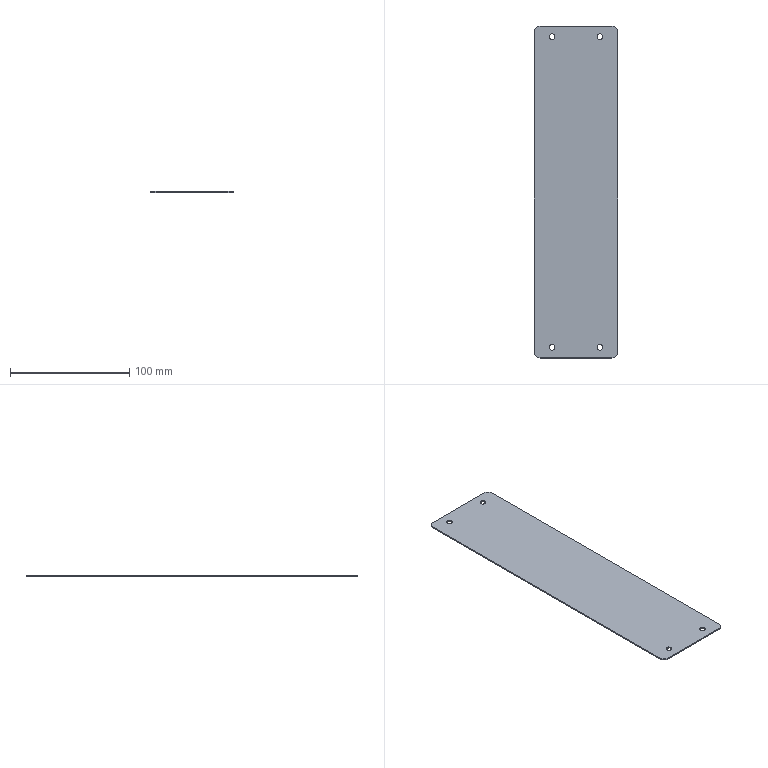Part | SolidWorks | features BreakCorner 1, FlatPattern 1, HoleWzd 1, SMBaseFlange 1, SheetMetal 1 | 1 solid | 18 faces | box 70 x 278 x 1 mm | volume 19366 mm3 | cylinder 12 | plane 6 | commonest cylinder face diameters 4.8 x8 10 x4
STEP:
#1=CARTESIAN_POINT('',(20.,127.6,0.));
#2=VERTEX_POINT('',#1);
#3=CARTESIAN_POINT('',(20.,132.4,0.));
#4=VERTEX_POINT('',#3);
#5=CARTESIAN_POINT('',(20.,130.,0.));
#6=DIRECTION('',(0.,0.,-1.));
#7=DIRECTION('',(0.,1.,0.));
#8=AXIS2_PLACEMENT_3D('',#5,#6,#7);
#9=CIRCLE('',#8,2.4);
#10=EDGE_CURVE('',#2,#4,#9,.T.);
#11=ORIENTED_EDGE('',*,*,#10,.F.);
#12=CARTESIAN_POINT('',(20.,127.6,-1.));
#13=VERTEX_POINT('',#12);
#14=CARTESIAN_POINT('',(20.,127.6,-1.));
#15=DIRECTION('',(0.,0.,-1.));
#16=VECTOR('',#15,1000.);
#17=LINE('',#14,#16);
#18=EDGE_CURVE('',#2,#13,#17,.T.);
#19=ORIENTED_EDGE('',*,*,#18,.T.);
#20=CARTESIAN_POINT('',(20.,132.4,-1.));
#21=VERTEX_POINT('',#20);
#22=CARTESIAN_POINT('',(20.,130.,-1.));
#23=DIRECTION('',(0.,0.,-1.));
#24=DIRECTION('',(0.,1.,0.));
#25=AXIS2_PLACEMENT_3D('',#22,#23,#24);
#26=CIRCLE('',#25,2.4);
#27=EDGE_CURVE('',#13,#21,#26,.T.);
#28=ORIENTED_EDGE('',*,*,#27,.T.);
#29=CARTESIAN_POINT('',(20.,132.4,-1.));
#30=DIRECTION('',(0.,0.,-1.));
#31=VECTOR('',#30,1000.);
#32=LINE('',#29,#31);
#33=EDGE_CURVE('',#4,#21,#32,.T.);
#34=ORIENTED_EDGE('',*,*,#33,.F.);
#35=EDGE_LOOP('',(#11,#19,#28,#34));
#36=FACE_OUTER_BOUND('',#35,.T.);
#37=CARTESIAN_POINT('',(20.,130.,-1.));
#38=DIRECTION('',(0.,0.,-1.));
#39=DIRECTION('',(0.,1.,0.));
#40=AXIS2_PLACEMENT_3D('',#37,#38,#39);
#41=CYLINDRICAL_SURFACE('',#40,2.4);
#42=ADVANCED_FACE('',(#36),#41,.F.);
#43=CARTESIAN_POINT('',(-20.,127.6,0.));
#44=VERTEX_POINT('',#43);
#45=CARTESIAN_POINT('',(-20.,132.4,0.));
#46=VERTEX_POINT('',#45);
#47=CARTESIAN_POINT('',(-20.,130.,0.));
#48=DIRECTION('',(0.,0.,-1.));
#49=DIRECTION('',(0.,1.,0.));
#50=AXIS2_PLACEMENT_3D('',#47,#48,#49);
#51=CIRCLE('',#50,2.4);
#52=EDGE_CURVE('',#44,#46,#51,.T.);
#53=ORIENTED_EDGE('',*,*,#52,.F.);
#54=CARTESIAN_POINT('',(-20.,127.6,-1.));
#55=VERTEX_POINT('',#54);
#56=CARTESIAN_POINT('',(-20.,127.6,-1.));
#57=DIRECTION('',(0.,0.,-1.));
#58=VECTOR('',#57,1000.);
#59=LINE('',#56,#58);
#60=EDGE_CURVE('',#44,#55,#59,.T.);
#61=ORIENTED_EDGE('',*,*,#60,.T.);
#62=CARTESIAN_POINT('',(-20.,132.4,-1.));
#63=VERTEX_POINT('',#62);
#64=CARTESIAN_POINT('',(-20.,130.,-1.));
#65=DIRECTION('',(0.,0.,-1.));
#66=DIRECTION('',(0.,1.,0.));
#67=AXIS2_PLACEMENT_3D('',#64,#65,#66);
#68=CIRCLE('',#67,2.4);
#69=EDGE_CURVE('',#55,#63,#68,.T.);
#70=ORIENTED_EDGE('',*,*,#69,.T.);
#71=CARTESIAN_POINT('',(-20.,132.4,-1.));
#72=DIRECTION('',(0.,0.,-1.));
#73=VECTOR('',#72,1000.);
#74=LINE('',#71,#73);
#75=EDGE_CURVE('',#46,#63,#74,.T.);
#76=ORIENTED_EDGE('',*,*,#75,.F.);
#77=EDGE_LOOP('',(#53,#61,#70,#76));
#78=FACE_OUTER_BOUND('',#77,.T.);
#79=CARTESIAN_POINT('',(-20.,130.,-1.));
#80=DIRECTION('',(0.,0.,-1.));
#81=DIRECTION('',(0.,1.,0.));
#82=AXIS2_PLACEMENT_3D('',#79,#80,#81);
#83=CYLINDRICAL_SURFACE('',#82,2.4);
#84=ADVANCED_FACE('',(#78),#83,.F.);
#85=CARTESIAN_POINT('',(20.,-132.4,0.));
#86=VERTEX_POINT('',#85);
#87=CARTESIAN_POINT('',(20.,-127.6,0.));
#88=VERTEX_POINT('',#87);
#89=CARTESIAN_POINT('',(20.,-130.,0.));
#90=DIRECTION('',(0.,0.,-1.));
#91=DIRECTION('',(0.,1.,0.));
#92=AXIS2_PLACEMENT_3D('',#89,#90,#91);
#93=CIRCLE('',#92,2.4);
#94=EDGE_CURVE('',#86,#88,#93,.T.);
#95=ORIENTED_EDGE('',*,*,#94,.F.);
#96=CARTESIAN_POINT('',(20.,-132.4,-1.));
#97=VERTEX_POINT('',#96);
#98=CARTESIAN_POINT('',(20.,-132.4,-1.));
#99=DIRECTION('',(0.,0.,-1.));
#100=VECTOR('',#99,1000.);
#101=LINE('',#98,#100);
#102=EDGE_CURVE('',#86,#97,#101,.T.);
#103=ORIENTED_EDGE('',*,*,#102,.T.);
#104=CARTESIAN_POINT('',(20.,-127.6,-1.));
#105=VERTEX_POINT('',#104);
#106=CARTESIAN_POINT('',(20.,-130.,-1.));
#107=DIRECTION('',(0.,0.,-1.));
#108=DIRECTION('',(0.,1.,0.));
#109=AXIS2_PLACEMENT_3D('',#106,#107,#108);
#110=CIRCLE('',#109,2.4);
#111=EDGE_CURVE('',#97,#105,#110,.T.);
#112=ORIENTED_EDGE('',*,*,#111,.T.);
#113=CARTESIAN_POINT('',(20.,-127.6,-1.));
#114=DIRECTION('',(0.,0.,-1.));
#115=VECTOR('',#114,1000.);
#116=LINE('',#113,#115);
#117=EDGE_CURVE('',#88,#105,#116,.T.);
#118=ORIENTED_EDGE('',*,*,#117,.F.);
#119=EDGE_LOOP('',(#95,#103,#112,#118));
#120=FACE_OUTER_BOUND('',#119,.T.);
#121=CARTESIAN_POINT('',(20.,-130.,-1.));
#122=DIRECTION('',(0.,0.,-1.));
#123=DIRECTION('',(0.,1.,0.));
#124=AXIS2_PLACEMENT_3D('',#121,#122,#123);
#125=CYLINDRICAL_SURFACE('',#124,2.4);
#126=ADVANCED_FACE('',(#120),#125,.F.);
#127=CARTESIAN_POINT('',(-20.,-132.4,0.));
#128=VERTEX_POINT('',#127);
#129=CARTESIAN_POINT('',(-20.,-127.6,0.));
#130=VERTEX_POINT('',#129);
#131=CARTESIAN_POINT('',(-20.,-130.,0.));
#132=DIRECTION('',(0.,0.,-1.));
#133=DIRECTION('',(0.,1.,0.));
#134=AXIS2_PLACEMENT_3D('',#131,#132,#133);
#135=CIRCLE('',#134,2.4);
#136=EDGE_CURVE('',#128,#130,#135,.T.);
#137=ORIENTED_EDGE('',*,*,#136,.F.);
#138=CARTESIAN_POINT('',(-20.,-132.4,-1.));
#139=VERTEX_POINT('',#138);
#140=CARTESIAN_POINT('',(-20.,-132.4,-1.));
#141=DIRECTION('',(0.,0.,-1.));
#142=VECTOR('',#141,1000.);
#143=LINE('',#140,#142);
#144=EDGE_CURVE('',#128,#139,#143,.T.);
#145=ORIENTED_EDGE('',*,*,#144,.T.);
#146=CARTESIAN_POINT('',(-20.,-127.6,-1.));
#147=VERTEX_POINT('',#146);
#148=CARTESIAN_POINT('',(-20.,-130.,-1.));
#149=DIRECTION('',(0.,0.,-1.));
#150=DIRECTION('',(0.,1.,0.));
#151=AXIS2_PLACEMENT_3D('',#148,#149,#150);
#152=CIRCLE('',#151,2.4);
#153=EDGE_CURVE('',#139,#147,#152,.T.);
#154=ORIENTED_EDGE('',*,*,#153,.T.);
#155=CARTESIAN_POINT('',(-20.,-127.6,-1.));
#156=DIRECTION('',(0.,0.,-1.));
#157=VECTOR('',#156,1000.);
#158=LINE('',#155,#157);
#159=EDGE_CURVE('',#130,#147,#158,.T.);
#160=ORIENTED_EDGE('',*,*,#159,.F.);
#161=EDGE_LOOP('',(#137,#145,#154,#160));
#162=FACE_OUTER_BOUND('',#161,.T.);
#163=CARTESIAN_POINT('',(-20.,-130.,-1.));
#164=DIRECTION('',(0.,0.,-1.));
#165=DIRECTION('',(0.,1.,0.));
#166=AXIS2_PLACEMENT_3D('',#163,#164,#165);
#167=CYLINDRICAL_SURFACE('',#166,2.4);
#168=ADVANCED_FACE('',(#162),#167,.F.);
#169=CARTESIAN_POINT('',(35.,-134.,-1.));
#170=VERTEX_POINT('',#169);
#171=CARTESIAN_POINT('',(35.,134.,-1.));
#172=VERTEX_POINT('',#171);
#173=CARTESIAN_POINT('',(35.,-139.,-1.));
#174=DIRECTION('',(0.,1.,0.));
#175=VECTOR('',#174,1000.);
#176=LINE('',#173,#175);
#177=EDGE_CURVE('',#170,#172,#176,.T.);
#178=ORIENTED_EDGE('',*,*,#177,.T.);
#179=CARTESIAN_POINT('',(35.,134.,0.));
#180=VERTEX_POINT('',#179);
#181=CARTESIAN_POINT('',(35.,134.,-1.));
#182=DIRECTION('',(0.,0.,1.));
#183=VECTOR('',#182,1000.);
#184=LINE('',#181,#183);
#185=EDGE_CURVE('',#172,#180,#184,.T.);
#186=ORIENTED_EDGE('',*,*,#185,.T.);
#187=CARTESIAN_POINT('',(35.,-134.,0.));
#188=VERTEX_POINT('',#187);
#189=CARTESIAN_POINT('',(35.,-139.,0.));
#190=DIRECTION('',(0.,1.,0.));
#191=VECTOR('',#190,1000.);
#192=LINE('',#189,#191);
#193=EDGE_CURVE('',#188,#180,#192,.T.);
#194=ORIENTED_EDGE('',*,*,#193,.F.);
#195=CARTESIAN_POINT('',(35.,-134.,-1.));
#196=DIRECTION('',(0.,0.,-1.));
#197=VECTOR('',#196,1000.);
#198=LINE('',#195,#197);
#199=EDGE_CURVE('',#188,#170,#198,.T.);
#200=ORIENTED_EDGE('',*,*,#199,.T.);
#201=EDGE_LOOP('',(#178,#186,#194,#200));
#202=FACE_OUTER_BOUND('',#201,.T.);
#203=CARTESIAN_POINT('',(35.,-139.,-1.));
#204=DIRECTION('',(1.,0.,0.));
#205=DIRECTION('',(0.,0.,-1.));
#206=AXIS2_PLACEMENT_3D('',#203,#204,#205);
#207=PLANE('',#206);
#208=ADVANCED_FACE('',(#202),#207,.T.);
#209=CARTESIAN_POINT('',(-30.,-139.,0.));
#210=VERTEX_POINT('',#209);
#211=CARTESIAN_POINT('',(30.,-139.,0.));
#212=VERTEX_POINT('',#211);
#213=CARTESIAN_POINT('',(-35.,-139.,0.));
#214=DIRECTION('',(1.,0.,0.));
#215=VECTOR('',#214,1000.);
#216=LINE('',#213,#215);
#217=EDGE_CURVE('',#210,#212,#216,.T.);
#218=ORIENTED_EDGE('',*,*,#217,.F.);
#219=CARTESIAN_POINT('',(-30.,-139.,-1.));
#220=VERTEX_POINT('',#219);
#221=CARTESIAN_POINT('',(-30.,-139.,-1.));
#222=DIRECTION('',(0.,0.,-1.));
#223=VECTOR('',#222,1000.);
#224=LINE('',#221,#223);
#225=EDGE_CURVE('',#210,#220,#224,.T.);
#226=ORIENTED_EDGE('',*,*,#225,.T.);
#227=CARTESIAN_POINT('',(30.,-139.,-1.));
#228=VERTEX_POINT('',#227);
#229=CARTESIAN_POINT('',(-35.,-139.,-1.));
#230=DIRECTION('',(1.,0.,0.));
#231=VECTOR('',#230,1000.);
#232=LINE('',#229,#231);
#233=EDGE_CURVE('',#220,#228,#232,.T.);
#234=ORIENTED_EDGE('',*,*,#233,.T.);
#235=CARTESIAN_POINT('',(30.,-139.,-1.));
#236=DIRECTION('',(0.,0.,1.));
#237=VECTOR('',#236,1000.);
#238=LINE('',#235,#237);
#239=EDGE_CURVE('',#228,#212,#238,.T.);
#240=ORIENTED_EDGE('',*,*,#239,.T.);
#241=EDGE_LOOP('',(#218,#226,#234,#240));
#242=FACE_OUTER_BOUND('',#241,.T.);
#243=CARTESIAN_POINT('',(-35.,-139.,-1.));
#244=DIRECTION('',(0.,-1.,0.));
#245=DIRECTION('',(0.,0.,-1.));
#246=AXIS2_PLACEMENT_3D('',#243,#244,#245);
#247=PLANE('',#246);
#248=ADVANCED_FACE('',(#242),#247,.T.);
#249=CARTESIAN_POINT('',(-35.,134.,0.));
#250=VERTEX_POINT('',#249);
#251=CARTESIAN_POINT('',(-35.,-134.,0.));
#252=VERTEX_POINT('',#251);
#253=CARTESIAN_POINT('',(-35.,-139.,0.));
#254=DIRECTION('',(0.,-1.,0.));
#255=VECTOR('',#254,1000.);
#256=LINE('',#253,#255);
#257=EDGE_CURVE('',#250,#252,#256,.T.);
#258=ORIENTED_EDGE('',*,*,#257,.F.);
#259=CARTESIAN_POINT('',(-35.,134.,-1.));
#260=VERTEX_POINT('',#259);
#261=CARTESIAN_POINT('',(-35.,134.,-1.));
#262=DIRECTION('',(0.,0.,-1.));
#263=VECTOR('',#262,1000.);
#264=LINE('',#261,#263);
#265=EDGE_CURVE('',#250,#260,#264,.T.);
#266=ORIENTED_EDGE('',*,*,#265,.T.);
#267=CARTESIAN_POINT('',(-35.,-134.,-1.));
#268=VERTEX_POINT('',#267);
#269=CARTESIAN_POINT('',(-35.,-139.,-1.));
#270=DIRECTION('',(0.,-1.,0.));
#271=VECTOR('',#270,1000.);
#272=LINE('',#269,#271);
#273=EDGE_CURVE('',#260,#268,#272,.T.);
#274=ORIENTED_EDGE('',*,*,#273,.T.);
#275=CARTESIAN_POINT('',(-35.,-134.,-1.));
#276=DIRECTION('',(0.,0.,1.));
#277=VECTOR('',#276,1000.);
#278=LINE('',#275,#277);
#279=EDGE_CURVE('',#268,#252,#278,.T.);
#280=ORIENTED_EDGE('',*,*,#279,.T.);
#281=EDGE_LOOP('',(#258,#266,#274,#280));
#282=FACE_OUTER_BOUND('',#281,.T.);
#283=CARTESIAN_POINT('',(-35.,-139.,-1.));
#284=DIRECTION('',(-1.,0.,0.));
#285=DIRECTION('',(0.,0.,1.));
#286=AXIS2_PLACEMENT_3D('',#283,#284,#285);
#287=PLANE('',#286);
#288=ADVANCED_FACE('',(#282),#287,.T.);
#289=CARTESIAN_POINT('',(30.,139.,0.));
#290=VERTEX_POINT('',#289);
#291=CARTESIAN_POINT('',(-30.,139.,0.));
#292=VERTEX_POINT('',#291);
#293=CARTESIAN_POINT('',(-35.,139.,0.));
#294=DIRECTION('',(-1.,0.,0.));
#295=VECTOR('',#294,1000.);
#296=LINE('',#293,#295);
#297=EDGE_CURVE('',#290,#292,#296,.T.);
#298=ORIENTED_EDGE('',*,*,#297,.F.);
#299=CARTESIAN_POINT('',(30.,139.,-1.));
#300=VERTEX_POINT('',#299);
#301=CARTESIAN_POINT('',(30.,139.,-1.));
#302=DIRECTION('',(0.,0.,-1.));
#303=VECTOR('',#302,1000.);
#304=LINE('',#301,#303);
#305=EDGE_CURVE('',#290,#300,#304,.T.);
#306=ORIENTED_EDGE('',*,*,#305,.T.);
#307=CARTESIAN_POINT('',(-30.,139.,-1.));
#308=VERTEX_POINT('',#307);
#309=CARTESIAN_POINT('',(-35.,139.,-1.));
#310=DIRECTION('',(-1.,0.,0.));
#311=VECTOR('',#310,1000.);
#312=LINE('',#309,#311);
#313=EDGE_CURVE('',#300,#308,#312,.T.);
#314=ORIENTED_EDGE('',*,*,#313,.T.);
#315=CARTESIAN_POINT('',(-30.,139.,-1.));
#316=DIRECTION('',(0.,0.,1.));
#317=VECTOR('',#316,1000.);
#318=LINE('',#315,#317);
#319=EDGE_CURVE('',#308,#292,#318,.T.);
#320=ORIENTED_EDGE('',*,*,#319,.T.);
#321=EDGE_LOOP('',(#298,#306,#314,#320));
#322=FACE_OUTER_BOUND('',#321,.T.);
#323=CARTESIAN_POINT('',(-35.,139.,-1.));
#324=DIRECTION('',(0.,1.,0.));
#325=DIRECTION('',(0.,0.,1.));
#326=AXIS2_PLACEMENT_3D('',#323,#324,#325);
#327=PLANE('',#326);
#328=ADVANCED_FACE('',(#322),#327,.T.);
#329=CARTESIAN_POINT('',(20.,130.,-1.));
#330=DIRECTION('',(0.,0.,-1.));
#331=DIRECTION('',(0.,1.,0.));
#332=AXIS2_PLACEMENT_3D('',#329,#330,#331);
#333=CIRCLE('',#332,2.4);
#334=EDGE_CURVE('',#21,#13,#333,.T.);
#335=ORIENTED_EDGE('',*,*,#334,.F.);
#336=ORIENTED_EDGE('',*,*,#27,.F.);
#337=EDGE_LOOP('',(#335,#336));
#338=FACE_BOUND('',#337,.T.);
#339=CARTESIAN_POINT('',(-20.,130.,-1.));
#340=DIRECTION('',(0.,0.,-1.));
#341=DIRECTION('',(0.,1.,0.));
#342=AXIS2_PLACEMENT_3D('',#339,#340,#341);
#343=CIRCLE('',#342,2.4);
#344=EDGE_CURVE('',#63,#55,#343,.T.);
#345=ORIENTED_EDGE('',*,*,#344,.F.);
#346=ORIENTED_EDGE('',*,*,#69,.F.);
#347=EDGE_LOOP('',(#345,#346));
#348=FACE_BOUND('',#347,.T.);
#349=CARTESIAN_POINT('',(20.,-130.,-1.));
#350=DIRECTION('',(0.,0.,-1.));
#351=DIRECTION('',(0.,1.,0.));
#352=AXIS2_PLACEMENT_3D('',#349,#350,#351);
#353=CIRCLE('',#352,2.4);
#354=EDGE_CURVE('',#105,#97,#353,.T.);
#355=ORIENTED_EDGE('',*,*,#354,.F.);
#356=ORIENTED_EDGE('',*,*,#111,.F.);
#357=EDGE_LOOP('',(#355,#356));
#358=FACE_BOUND('',#357,.T.);
#359=CARTESIAN_POINT('',(-20.,-130.,-1.));
#360=DIRECTION('',(0.,0.,-1.));
#361=DIRECTION('',(0.,1.,0.));
#362=AXIS2_PLACEMENT_3D('',#359,#360,#361);
#363=CIRCLE('',#362,2.4);
#364=EDGE_CURVE('',#147,#139,#363,.T.);
#365=ORIENTED_EDGE('',*,*,#364,.F.);
#366=ORIENTED_EDGE('',*,*,#153,.F.);
#367=EDGE_LOOP('',(#365,#366));
#368=FACE_BOUND('',#367,.T.);
#369=ORIENTED_EDGE('',*,*,#313,.F.);
#370=CARTESIAN_POINT('',(30.,134.,-1.));
#371=DIRECTION('',(0.,0.,-1.));
#372=DIRECTION('',(-1.,0.,0.));
#373=AXIS2_PLACEMENT_3D('',#370,#371,#372);
#374=CIRCLE('',#373,5.);
#375=EDGE_CURVE('',#300,#172,#374,.T.);
#376=ORIENTED_EDGE('',*,*,#375,.T.);
#377=ORIENTED_EDGE('',*,*,#177,.F.);
#378=CARTESIAN_POINT('',(30.,-134.,-1.));
#379=DIRECTION('',(0.,0.,-1.));
#380=DIRECTION('',(-1.,0.,0.));
#381=AXIS2_PLACEMENT_3D('',#378,#379,#380);
#382=CIRCLE('',#381,5.);
#383=EDGE_CURVE('',#170,#228,#382,.T.);
#384=ORIENTED_EDGE('',*,*,#383,.T.);
#385=ORIENTED_EDGE('',*,*,#233,.F.);
#386=CARTESIAN_POINT('',(-30.,-134.,-1.));
#387=DIRECTION('',(0.,0.,-1.));
#388=DIRECTION('',(-1.,0.,0.));
#389=AXIS2_PLACEMENT_3D('',#386,#387,#388);
#390=CIRCLE('',#389,5.);
#391=EDGE_CURVE('',#220,#268,#390,.T.);
#392=ORIENTED_EDGE('',*,*,#391,.T.);
#393=ORIENTED_EDGE('',*,*,#273,.F.);
#394=CARTESIAN_POINT('',(-30.,134.,-1.));
#395=DIRECTION('',(0.,0.,-1.));
#396=DIRECTION('',(-1.,0.,0.));
#397=AXIS2_PLACEMENT_3D('',#394,#395,#396);
#398=CIRCLE('',#397,5.);
#399=EDGE_CURVE('',#260,#308,#398,.T.);
#400=ORIENTED_EDGE('',*,*,#399,.T.);
#401=EDGE_LOOP('',(#369,#376,#377,#384,#385,#392,#393,#400));
#402=FACE_OUTER_BOUND('',#401,.T.);
#403=CARTESIAN_POINT('',(0.,0.,-1.));
#404=DIRECTION('',(0.,0.,-1.));
#405=DIRECTION('',(-1.,0.,0.));
#406=AXIS2_PLACEMENT_3D('',#403,#404,#405);
#407=PLANE('',#406);
#408=ADVANCED_FACE('',(#338,#348,#358,#368,#402),#407,.T.);
#409=CARTESIAN_POINT('',(20.,130.,0.));
#410=DIRECTION('',(0.,0.,-1.));
#411=DIRECTION('',(0.,1.,0.));
#412=AXIS2_PLACEMENT_3D('',#409,#410,#411);
#413=CIRCLE('',#412,2.4);
#414=EDGE_CURVE('',#4,#2,#413,.T.);
#415=ORIENTED_EDGE('',*,*,#414,.T.);
#416=ORIENTED_EDGE('',*,*,#10,.T.);
#417=EDGE_LOOP('',(#415,#416));
#418=FACE_BOUND('',#417,.T.);
#419=CARTESIAN_POINT('',(-20.,130.,0.));
#420=DIRECTION('',(0.,0.,-1.));
#421=DIRECTION('',(0.,1.,0.));
#422=AXIS2_PLACEMENT_3D('',#419,#420,#421);
#423=CIRCLE('',#422,2.4);
#424=EDGE_CURVE('',#46,#44,#423,.T.);
#425=ORIENTED_EDGE('',*,*,#424,.T.);
#426=ORIENTED_EDGE('',*,*,#52,.T.);
#427=EDGE_LOOP('',(#425,#426));
#428=FACE_BOUND('',#427,.T.);
#429=CARTESIAN_POINT('',(20.,-130.,0.));
#430=DIRECTION('',(0.,0.,-1.));
#431=DIRECTION('',(0.,1.,0.));
#432=AXIS2_PLACEMENT_3D('',#429,#430,#431);
#433=CIRCLE('',#432,2.4);
#434=EDGE_CURVE('',#88,#86,#433,.T.);
#435=ORIENTED_EDGE('',*,*,#434,.T.);
#436=ORIENTED_EDGE('',*,*,#94,.T.);
#437=EDGE_LOOP('',(#435,#436));
#438=FACE_BOUND('',#437,.T.);
#439=CARTESIAN_POINT('',(-20.,-130.,0.));
#440=DIRECTION('',(0.,0.,-1.));
#441=DIRECTION('',(0.,1.,0.));
#442=AXIS2_PLACEMENT_3D('',#439,#440,#441);
#443=CIRCLE('',#442,2.4);
#444=EDGE_CURVE('',#130,#128,#443,.T.);
#445=ORIENTED_EDGE('',*,*,#444,.T.);
#446=ORIENTED_EDGE('',*,*,#136,.T.);
#447=EDGE_LOOP('',(#445,#446));
#448=FACE_BOUND('',#447,.T.);
#449=ORIENTED_EDGE('',*,*,#193,.T.);
#450=CARTESIAN_POINT('',(30.,134.,0.));
#451=DIRECTION('',(0.,0.,1.));
#452=DIRECTION('',(-1.,0.,0.));
#453=AXIS2_PLACEMENT_3D('',#450,#451,#452);
#454=CIRCLE('',#453,5.);
#455=EDGE_CURVE('',#180,#290,#454,.T.);
#456=ORIENTED_EDGE('',*,*,#455,.T.);
#457=ORIENTED_EDGE('',*,*,#297,.T.);
#458=CARTESIAN_POINT('',(-30.,134.,0.));
#459=DIRECTION('',(0.,0.,1.));
#460=DIRECTION('',(-1.,0.,0.));
#461=AXIS2_PLACEMENT_3D('',#458,#459,#460);
#462=CIRCLE('',#461,5.);
#463=EDGE_CURVE('',#292,#250,#462,.T.);
#464=ORIENTED_EDGE('',*,*,#463,.T.);
#465=ORIENTED_EDGE('',*,*,#257,.T.);
#466=CARTESIAN_POINT('',(-30.,-134.,0.));
#467=DIRECTION('',(0.,0.,1.));
#468=DIRECTION('',(-1.,0.,0.));
#469=AXIS2_PLACEMENT_3D('',#466,#467,#468);
#470=CIRCLE('',#469,5.);
#471=EDGE_CURVE('',#252,#210,#470,.T.);
#472=ORIENTED_EDGE('',*,*,#471,.T.);
#473=ORIENTED_EDGE('',*,*,#217,.T.);
#474=CARTESIAN_POINT('',(30.,-134.,0.));
#475=DIRECTION('',(0.,0.,1.));
#476=DIRECTION('',(-1.,0.,0.));
#477=AXIS2_PLACEMENT_3D('',#474,#475,#476);
#478=CIRCLE('',#477,5.);
#479=EDGE_CURVE('',#212,#188,#478,.T.);
#480=ORIENTED_EDGE('',*,*,#479,.T.);
#481=EDGE_LOOP('',(#449,#456,#457,#464,#465,#472,#473,#480));
#482=FACE_OUTER_BOUND('',#481,.T.);
#483=CARTESIAN_POINT('',(0.,0.,0.));
#484=DIRECTION('',(0.,0.,-1.));
#485=DIRECTION('',(-1.,0.,0.));
#486=AXIS2_PLACEMENT_3D('',#483,#484,#485);
#487=PLANE('',#486);
#488=ADVANCED_FACE('',(#418,#428,#438,#448,#482),#487,.F.);
#489=ORIENTED_EDGE('',*,*,#144,.F.);
#490=ORIENTED_EDGE('',*,*,#444,.F.);
#491=ORIENTED_EDGE('',*,*,#159,.T.);
#492=ORIENTED_EDGE('',*,*,#364,.T.);
#493=EDGE_LOOP('',(#489,#490,#491,#492));
#494=FACE_OUTER_BOUND('',#493,.T.);
#495=CARTESIAN_POINT('',(-20.,-130.,-1.));
#496=DIRECTION('',(0.,0.,-1.));
#497=DIRECTION('',(0.,1.,0.));
#498=AXIS2_PLACEMENT_3D('',#495,#496,#497);
#499=CYLINDRICAL_SURFACE('',#498,2.4);
#500=ADVANCED_FACE('',(#494),#499,.F.);
#501=ORIENTED_EDGE('',*,*,#102,.F.);
#502=ORIENTED_EDGE('',*,*,#434,.F.);
#503=ORIENTED_EDGE('',*,*,#117,.T.);
#504=ORIENTED_EDGE('',*,*,#354,.T.);
#505=EDGE_LOOP('',(#501,#502,#503,#504));
#506=FACE_OUTER_BOUND('',#505,.T.);
#507=CARTESIAN_POINT('',(20.,-130.,-1.));
#508=DIRECTION('',(0.,0.,-1.));
#509=DIRECTION('',(0.,1.,0.));
#510=AXIS2_PLACEMENT_3D('',#507,#508,#509);
#511=CYLINDRICAL_SURFACE('',#510,2.4);
#512=ADVANCED_FACE('',(#506),#511,.F.);
#513=ORIENTED_EDGE('',*,*,#60,.F.);
#514=ORIENTED_EDGE('',*,*,#424,.F.);
#515=ORIENTED_EDGE('',*,*,#75,.T.);
#516=ORIENTED_EDGE('',*,*,#344,.T.);
#517=EDGE_LOOP('',(#513,#514,#515,#516));
#518=FACE_OUTER_BOUND('',#517,.T.);
#519=CARTESIAN_POINT('',(-20.,130.,-1.));
#520=DIRECTION('',(0.,0.,-1.));
#521=DIRECTION('',(0.,1.,0.));
#522=AXIS2_PLACEMENT_3D('',#519,#520,#521);
#523=CYLINDRICAL_SURFACE('',#522,2.4);
#524=ADVANCED_FACE('',(#518),#523,.F.);
#525=ORIENTED_EDGE('',*,*,#18,.F.);
#526=ORIENTED_EDGE('',*,*,#414,.F.);
#527=ORIENTED_EDGE('',*,*,#33,.T.);
#528=ORIENTED_EDGE('',*,*,#334,.T.);
#529=EDGE_LOOP('',(#525,#526,#527,#528));
#530=FACE_OUTER_BOUND('',#529,.T.);
#531=CARTESIAN_POINT('',(20.,130.,-1.));
#532=DIRECTION('',(0.,0.,-1.));
#533=DIRECTION('',(0.,1.,0.));
#534=AXIS2_PLACEMENT_3D('',#531,#532,#533);
#535=CYLINDRICAL_SURFACE('',#534,2.4);
#536=ADVANCED_FACE('',(#530),#535,.F.);
#537=ORIENTED_EDGE('',*,*,#375,.F.);
#538=ORIENTED_EDGE('',*,*,#305,.F.);
#539=ORIENTED_EDGE('',*,*,#455,.F.);
#540=ORIENTED_EDGE('',*,*,#185,.F.);
#541=EDGE_LOOP('',(#537,#538,#539,#540));
#542=FACE_OUTER_BOUND('',#541,.T.);
#543=CARTESIAN_POINT('',(30.,134.,-1.));
#544=DIRECTION('',(0.,0.,1.));
#545=DIRECTION('',(1.,0.,0.));
#546=AXIS2_PLACEMENT_3D('',#543,#544,#545);
#547=CYLINDRICAL_SURFACE('',#546,5.);
#548=ADVANCED_FACE('',(#542),#547,.T.);
#549=ORIENTED_EDGE('',*,*,#399,.F.);
#550=ORIENTED_EDGE('',*,*,#265,.F.);
#551=ORIENTED_EDGE('',*,*,#463,.F.);
#552=ORIENTED_EDGE('',*,*,#319,.F.);
#553=EDGE_LOOP('',(#549,#550,#551,#552));
#554=FACE_OUTER_BOUND('',#553,.T.);
#555=CARTESIAN_POINT('',(-30.,134.,-1.));
#556=DIRECTION('',(0.,0.,1.));
#557=DIRECTION('',(1.,0.,0.));
#558=AXIS2_PLACEMENT_3D('',#555,#556,#557);
#559=CYLINDRICAL_SURFACE('',#558,5.);
#560=ADVANCED_FACE('',(#554),#559,.T.);
#561=ORIENTED_EDGE('',*,*,#391,.F.);
#562=ORIENTED_EDGE('',*,*,#225,.F.);
#563=ORIENTED_EDGE('',*,*,#471,.F.);
#564=ORIENTED_EDGE('',*,*,#279,.F.);
#565=EDGE_LOOP('',(#561,#562,#563,#564));
#566=FACE_OUTER_BOUND('',#565,.T.);
#567=CARTESIAN_POINT('',(-30.,-134.,-1.));
#568=DIRECTION('',(0.,0.,1.));
#569=DIRECTION('',(1.,0.,0.));
#570=AXIS2_PLACEMENT_3D('',#567,#568,#569);
#571=CYLINDRICAL_SURFACE('',#570,5.);
#572=ADVANCED_FACE('',(#566),#571,.T.);
#573=ORIENTED_EDGE('',*,*,#383,.F.);
#574=ORIENTED_EDGE('',*,*,#199,.F.);
#575=ORIENTED_EDGE('',*,*,#479,.F.);
#576=ORIENTED_EDGE('',*,*,#239,.F.);
#577=EDGE_LOOP('',(#573,#574,#575,#576));
#578=FACE_OUTER_BOUND('',#577,.T.);
#579=CARTESIAN_POINT('',(30.,-134.,-1.));
#580=DIRECTION('',(0.,0.,1.));
#581=DIRECTION('',(1.,0.,0.));
#582=AXIS2_PLACEMENT_3D('',#579,#580,#581);
#583=CYLINDRICAL_SURFACE('',#582,5.);
#584=ADVANCED_FACE('',(#578),#583,.T.);
#585=CLOSED_SHELL('',(#42,#84,#126,#168,#208,#248,#288,#328,#408,#488,#500,#512,#524,#536,#548,#560,#572,#584));
#586=MANIFOLD_SOLID_BREP('',#585);
#587=CARTESIAN_POINT('',(0.,0.,0.));
#588=DIRECTION('',(0.,0.,1.));
#589=DIRECTION('',(1.,0.,0.));
#590=AXIS2_PLACEMENT_3D('',#587,#588,#589);
#591=(LENGTH_UNIT()NAMED_UNIT(*)SI_UNIT(.MILLI.,.METRE.));
#592=UNCERTAINTY_MEASURE_WITH_UNIT(LENGTH_MEASURE(0.00001),#591,'','');
#593=(NAMED_UNIT(*)PLANE_ANGLE_UNIT()SI_UNIT($,.RADIAN.));
#594=(NAMED_UNIT(*)SI_UNIT($,.STERADIAN.)SOLID_ANGLE_UNIT());
#595=(GEOMETRIC_REPRESENTATION_CONTEXT(3)GLOBAL_UNCERTAINTY_ASSIGNED_CONTEXT((#592))GLOBAL_UNIT_ASSIGNED_CONTEXT((#591,#593,#594))REPRESENTATION_CONTEXT('',''));
#596=ADVANCED_BREP_SHAPE_REPRESENTATION('',(#586,#590),#595);